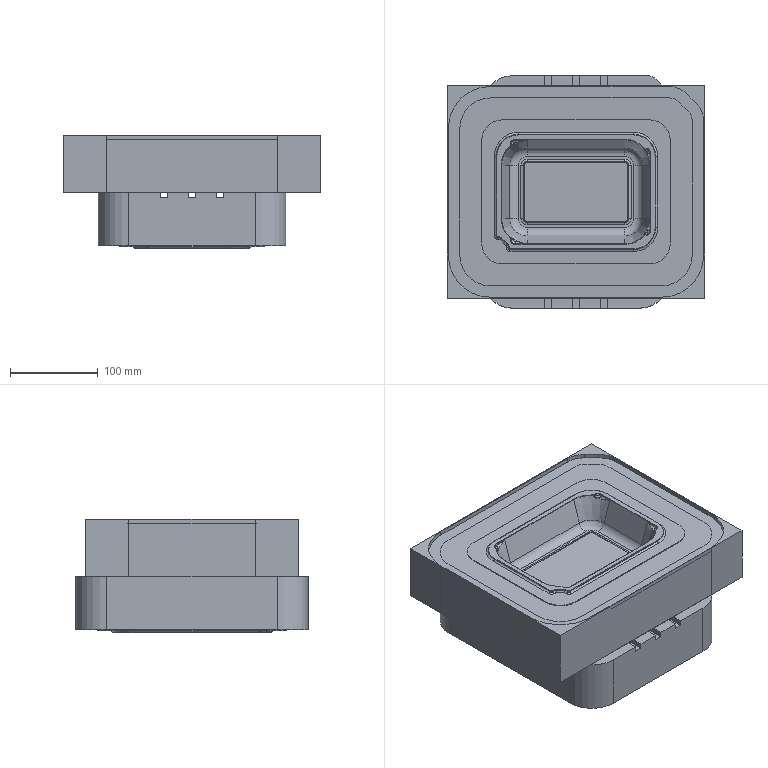Part | 4 solids | 607 faces | box 293.342 x 265.342 x 129.5 mm | volume 6624778 mm3 | plane 246 | cylinder 215 | spline 80 | torus 52 | cone 14 | commonest cylinder face diameters 2 x35 8 x35 1 x30 5.359 x16 5 x14 70 x9